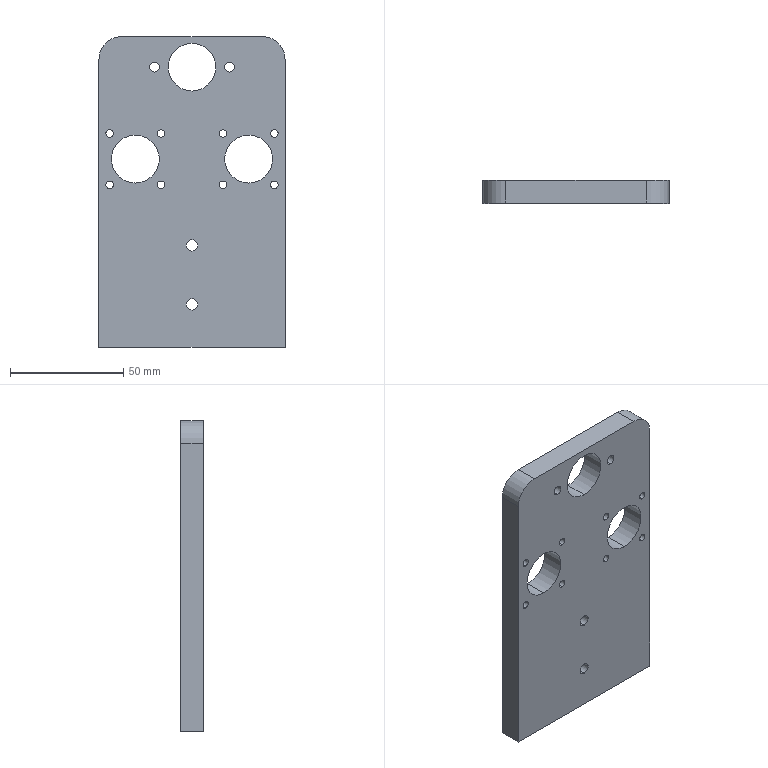Part | 1 solid | 60 faces | box 82 x 10 x 137 mm | volume 99019 mm3 | cylinder 44 | cone 8 | plane 8 | commonest cylinder face diameters 3.3 x20 5 x8 4.3 x4 8 x4 21.1 x4 20 x2